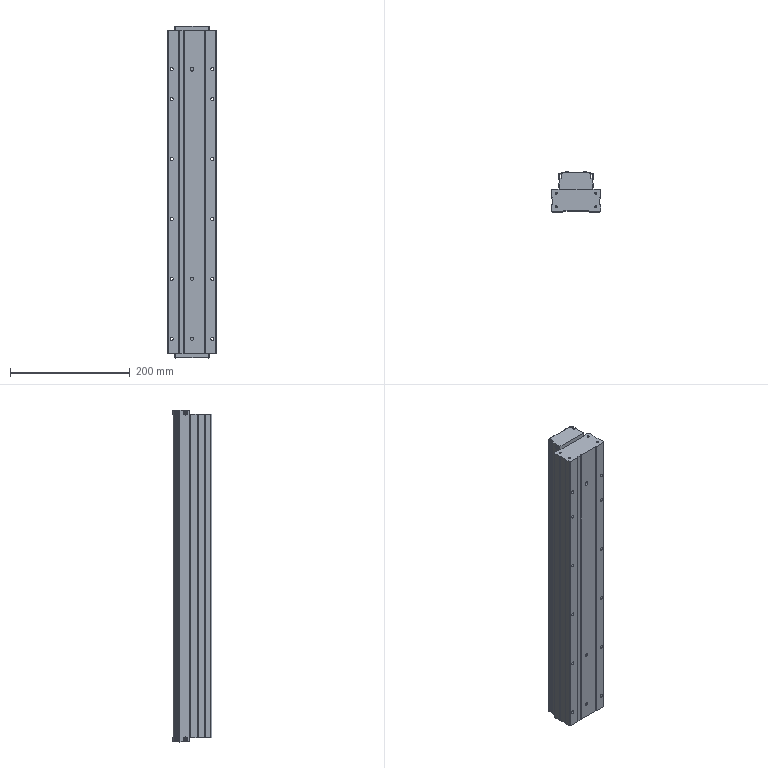Part | SolidWorks | features BaseBody 1 | 1 solid | 323 faces | box 82 x 66 x 554 mm | volume 2405342 mm3 | plane 156 | cylinder 135 | spline 16 | cone 16 | commonest cylinder face diameters 5.4 x24 2 x17 3.3 x16 6.7 x16 0.4 x14 1 x12